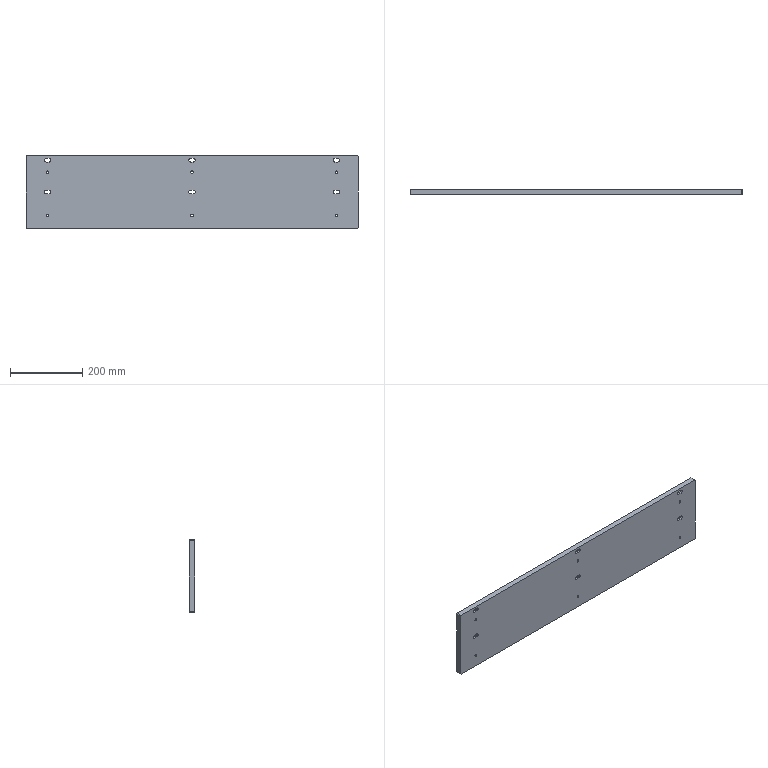Part | NX | features BREP 1 | 1 solid | 76 faces | box 920 x 15 x 200 mm | volume 2734881 mm3 | plane 40 | cylinder 36 | commonest cylinder face diameters 6.8 x12 10 x12 15 x12